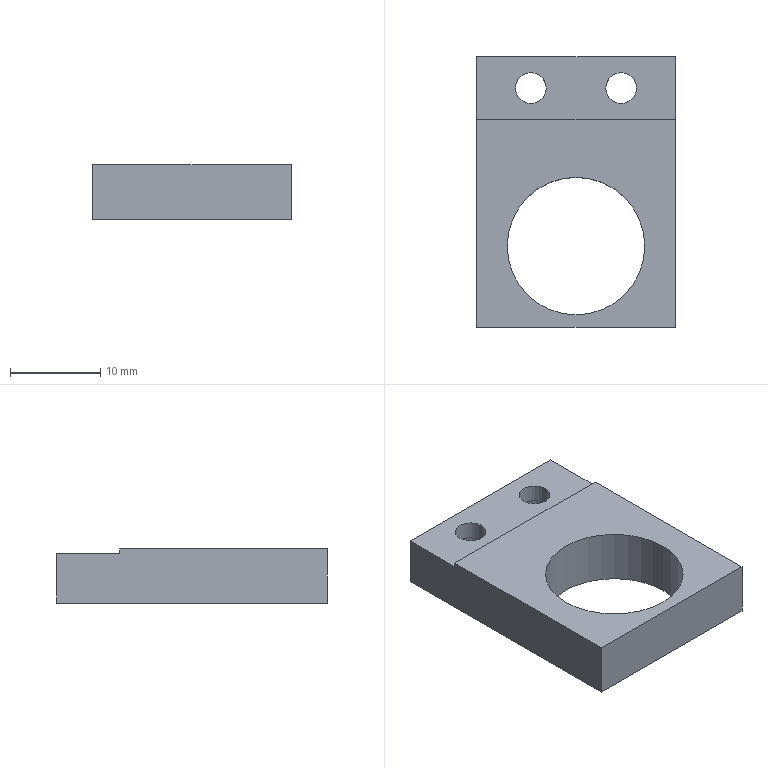Part | SolidWorks | features ICE 2, Extrusion 1 | 1 solid | 20 faces | box 22 x 30 x 6 mm | volume 2556 mm3 | cylinder 10 | plane 10 | commonest cylinder face diameters 3.4 x4 6 x4 15.23 x2
STEP:
#1=CARTESIAN_POINT('',(-0.003936,0.01062,0.0035));
#2=VERTEX_POINT('',#1);
#3=CARTESIAN_POINT('',(-0.009936,0.01062,0.0035));
#4=VERTEX_POINT('',#3);
#5=CARTESIAN_POINT('',(-0.006936,0.01062,0.0035));
#6=DIRECTION('',(0.,0.,-1.));
#7=DIRECTION('',(-1.,0.,0.));
#8=AXIS2_PLACEMENT_3D('',#5,#6,#7);
#9=CIRCLE('',#8,0.003);
#10=EDGE_CURVE('',#2,#4,#9,.T.);
#11=ORIENTED_EDGE('',*,*,#10,.F.);
#12=CARTESIAN_POINT('',(-0.003936,0.01062,0.));
#13=VERTEX_POINT('',#12);
#14=CARTESIAN_POINT('',(-0.003936,0.01062,0.0035));
#15=DIRECTION('',(0.,0.,-1.));
#16=VECTOR('',#15,1.);
#17=LINE('',#14,#16);
#18=EDGE_CURVE('',#2,#13,#17,.T.);
#19=ORIENTED_EDGE('',*,*,#18,.T.);
#20=CARTESIAN_POINT('',(-0.009936,0.01062,0.));
#21=VERTEX_POINT('',#20);
#22=CARTESIAN_POINT('',(-0.006936,0.01062,0.));
#23=DIRECTION('',(0.,0.,-1.));
#24=DIRECTION('',(-1.,0.,0.));
#25=AXIS2_PLACEMENT_3D('',#22,#23,#24);
#26=CIRCLE('',#25,0.003);
#27=EDGE_CURVE('',#13,#21,#26,.T.);
#28=ORIENTED_EDGE('',*,*,#27,.T.);
#29=CARTESIAN_POINT('',(-0.009936,0.01062,0.0035));
#30=DIRECTION('',(0.,0.,-1.));
#31=VECTOR('',#30,1.);
#32=LINE('',#29,#31);
#33=EDGE_CURVE('',#4,#21,#32,.T.);
#34=ORIENTED_EDGE('',*,*,#33,.F.);
#35=EDGE_LOOP('',(#11,#19,#28,#34));
#36=FACE_OUTER_BOUND('',#35,.T.);
#37=CARTESIAN_POINT('',(-0.006936,0.01062,0.0035));
#38=DIRECTION('',(0.,0.,-1.));
#39=DIRECTION('',(-1.,0.,0.));
#40=AXIS2_PLACEMENT_3D('',#37,#38,#39);
#41=CYLINDRICAL_SURFACE('',#40,0.003);
#42=ADVANCED_FACE('',(#36),#41,.F.);
#43=CARTESIAN_POINT('',(0.006064,0.01062,0.0035));
#44=VERTEX_POINT('',#43);
#45=CARTESIAN_POINT('',(0.00006422,0.01062,0.0035));
#46=VERTEX_POINT('',#45);
#47=CARTESIAN_POINT('',(0.003064,0.01062,0.0035));
#48=DIRECTION('',(0.,0.,-1.));
#49=DIRECTION('',(-1.,0.,0.));
#50=AXIS2_PLACEMENT_3D('',#47,#48,#49);
#51=CIRCLE('',#50,0.003);
#52=EDGE_CURVE('',#44,#46,#51,.T.);
#53=ORIENTED_EDGE('',*,*,#52,.F.);
#54=CARTESIAN_POINT('',(0.006064,0.01062,0.));
#55=VERTEX_POINT('',#54);
#56=CARTESIAN_POINT('',(0.006064,0.01062,0.0035));
#57=DIRECTION('',(0.,0.,-1.));
#58=VECTOR('',#57,1.);
#59=LINE('',#56,#58);
#60=EDGE_CURVE('',#44,#55,#59,.T.);
#61=ORIENTED_EDGE('',*,*,#60,.T.);
#62=CARTESIAN_POINT('',(0.00006422,0.01062,0.));
#63=VERTEX_POINT('',#62);
#64=CARTESIAN_POINT('',(0.003064,0.01062,0.));
#65=DIRECTION('',(0.,0.,-1.));
#66=DIRECTION('',(-1.,0.,0.));
#67=AXIS2_PLACEMENT_3D('',#64,#65,#66);
#68=CIRCLE('',#67,0.003);
#69=EDGE_CURVE('',#55,#63,#68,.T.);
#70=ORIENTED_EDGE('',*,*,#69,.T.);
#71=CARTESIAN_POINT('',(0.00006422,0.01062,0.0035));
#72=DIRECTION('',(0.,0.,-1.));
#73=VECTOR('',#72,1.);
#74=LINE('',#71,#73);
#75=EDGE_CURVE('',#46,#63,#74,.T.);
#76=ORIENTED_EDGE('',*,*,#75,.F.);
#77=EDGE_LOOP('',(#53,#61,#70,#76));
#78=FACE_OUTER_BOUND('',#77,.T.);
#79=CARTESIAN_POINT('',(0.003064,0.01062,0.0035));
#80=DIRECTION('',(0.,0.,-1.));
#81=DIRECTION('',(-1.,0.,0.));
#82=AXIS2_PLACEMENT_3D('',#79,#80,#81);
#83=CYLINDRICAL_SURFACE('',#82,0.003);
#84=ADVANCED_FACE('',(#78),#83,.F.);
#85=CARTESIAN_POINT('',(-0.009551,-0.006881,0.006));
#86=VERTEX_POINT('',#85);
#87=CARTESIAN_POINT('',(0.005679,-0.006881,0.006));
#88=VERTEX_POINT('',#87);
#89=CARTESIAN_POINT('',(-0.001936,-0.006881,0.006));
#90=DIRECTION('',(0.,0.,1.));
#91=DIRECTION('',(1.,0.,0.));
#92=AXIS2_PLACEMENT_3D('',#89,#90,#91);
#93=CIRCLE('',#92,0.007615);
#94=EDGE_CURVE('',#86,#88,#93,.T.);
#95=ORIENTED_EDGE('',*,*,#94,.T.);
#96=CARTESIAN_POINT('',(0.005679,-0.006881,0.));
#97=VERTEX_POINT('',#96);
#98=CARTESIAN_POINT('',(0.005679,-0.006881,0.006));
#99=DIRECTION('',(0.,0.,-1.));
#100=VECTOR('',#99,1.);
#101=LINE('',#98,#100);
#102=EDGE_CURVE('',#88,#97,#101,.T.);
#103=ORIENTED_EDGE('',*,*,#102,.T.);
#104=CARTESIAN_POINT('',(-0.009551,-0.006881,0.));
#105=VERTEX_POINT('',#104);
#106=CARTESIAN_POINT('',(-0.001936,-0.006881,0.));
#107=DIRECTION('',(0.,0.,1.));
#108=DIRECTION('',(1.,0.,0.));
#109=AXIS2_PLACEMENT_3D('',#106,#107,#108);
#110=CIRCLE('',#109,0.007615);
#111=EDGE_CURVE('',#105,#97,#110,.T.);
#112=ORIENTED_EDGE('',*,*,#111,.F.);
#113=CARTESIAN_POINT('',(-0.009551,-0.006881,0.006));
#114=DIRECTION('',(0.,0.,-1.));
#115=VECTOR('',#114,1.);
#116=LINE('',#113,#115);
#117=EDGE_CURVE('',#86,#105,#116,.T.);
#118=ORIENTED_EDGE('',*,*,#117,.F.);
#119=EDGE_LOOP('',(#95,#103,#112,#118));
#120=FACE_OUTER_BOUND('',#119,.T.);
#121=CARTESIAN_POINT('',(-0.001936,-0.006881,0.006));
#122=DIRECTION('',(0.,0.,-1.));
#123=DIRECTION('',(-1.,0.,0.));
#124=AXIS2_PLACEMENT_3D('',#121,#122,#123);
#125=CYLINDRICAL_SURFACE('',#124,0.007615);
#126=ADVANCED_FACE('',(#120),#125,.F.);
#127=CARTESIAN_POINT('',(0.004764,0.01062,0.0055));
#128=VERTEX_POINT('',#127);
#129=CARTESIAN_POINT('',(0.001364,0.01062,0.0055));
#130=VERTEX_POINT('',#129);
#131=CARTESIAN_POINT('',(0.003064,0.01062,0.0055));
#132=DIRECTION('',(0.,0.,-1.));
#133=DIRECTION('',(-1.,0.,0.));
#134=AXIS2_PLACEMENT_3D('',#131,#132,#133);
#135=CIRCLE('',#134,0.0017);
#136=EDGE_CURVE('',#128,#130,#135,.T.);
#137=ORIENTED_EDGE('',*,*,#136,.F.);
#138=CARTESIAN_POINT('',(0.004764,0.01062,0.0035));
#139=VERTEX_POINT('',#138);
#140=CARTESIAN_POINT('',(0.004764,0.01062,0.006));
#141=DIRECTION('',(0.,0.,-1.));
#142=VECTOR('',#141,1.);
#143=LINE('',#140,#142);
#144=EDGE_CURVE('',#128,#139,#143,.T.);
#145=ORIENTED_EDGE('',*,*,#144,.T.);
#146=CARTESIAN_POINT('',(0.001364,0.01062,0.0035));
#147=VERTEX_POINT('',#146);
#148=CARTESIAN_POINT('',(0.003064,0.01062,0.0035));
#149=DIRECTION('',(0.,0.,-1.));
#150=DIRECTION('',(-1.,0.,0.));
#151=AXIS2_PLACEMENT_3D('',#148,#149,#150);
#152=CIRCLE('',#151,0.0017);
#153=EDGE_CURVE('',#139,#147,#152,.T.);
#154=ORIENTED_EDGE('',*,*,#153,.T.);
#155=CARTESIAN_POINT('',(0.001364,0.01062,0.006));
#156=DIRECTION('',(0.,0.,-1.));
#157=VECTOR('',#156,1.);
#158=LINE('',#155,#157);
#159=EDGE_CURVE('',#130,#147,#158,.T.);
#160=ORIENTED_EDGE('',*,*,#159,.F.);
#161=EDGE_LOOP('',(#137,#145,#154,#160));
#162=FACE_OUTER_BOUND('',#161,.T.);
#163=CARTESIAN_POINT('',(0.003064,0.01062,0.006));
#164=DIRECTION('',(0.,0.,-1.));
#165=DIRECTION('',(-1.,0.,0.));
#166=AXIS2_PLACEMENT_3D('',#163,#164,#165);
#167=CYLINDRICAL_SURFACE('',#166,0.0017);
#168=ADVANCED_FACE('',(#162),#167,.F.);
#169=CARTESIAN_POINT('',(-0.005236,0.01062,0.0055));
#170=VERTEX_POINT('',#169);
#171=CARTESIAN_POINT('',(-0.008636,0.01062,0.0055));
#172=VERTEX_POINT('',#171);
#173=CARTESIAN_POINT('',(-0.006936,0.01062,0.0055));
#174=DIRECTION('',(0.,0.,-1.));
#175=DIRECTION('',(-1.,0.,0.));
#176=AXIS2_PLACEMENT_3D('',#173,#174,#175);
#177=CIRCLE('',#176,0.0017);
#178=EDGE_CURVE('',#170,#172,#177,.T.);
#179=ORIENTED_EDGE('',*,*,#178,.F.);
#180=CARTESIAN_POINT('',(-0.005236,0.01062,0.0035));
#181=VERTEX_POINT('',#180);
#182=CARTESIAN_POINT('',(-0.005236,0.01062,0.006));
#183=DIRECTION('',(0.,0.,-1.));
#184=VECTOR('',#183,1.);
#185=LINE('',#182,#184);
#186=EDGE_CURVE('',#170,#181,#185,.T.);
#187=ORIENTED_EDGE('',*,*,#186,.T.);
#188=CARTESIAN_POINT('',(-0.008636,0.01062,0.0035));
#189=VERTEX_POINT('',#188);
#190=CARTESIAN_POINT('',(-0.006936,0.01062,0.0035));
#191=DIRECTION('',(0.,0.,-1.));
#192=DIRECTION('',(-1.,0.,0.));
#193=AXIS2_PLACEMENT_3D('',#190,#191,#192);
#194=CIRCLE('',#193,0.0017);
#195=EDGE_CURVE('',#181,#189,#194,.T.);
#196=ORIENTED_EDGE('',*,*,#195,.T.);
#197=CARTESIAN_POINT('',(-0.008636,0.01062,0.006));
#198=DIRECTION('',(0.,0.,-1.));
#199=VECTOR('',#198,1.);
#200=LINE('',#197,#199);
#201=EDGE_CURVE('',#172,#189,#200,.T.);
#202=ORIENTED_EDGE('',*,*,#201,.F.);
#203=EDGE_LOOP('',(#179,#187,#196,#202));
#204=FACE_OUTER_BOUND('',#203,.T.);
#205=CARTESIAN_POINT('',(-0.006936,0.01062,0.006));
#206=DIRECTION('',(0.,0.,-1.));
#207=DIRECTION('',(-1.,0.,0.));
#208=AXIS2_PLACEMENT_3D('',#205,#206,#207);
#209=CYLINDRICAL_SURFACE('',#208,0.0017);
#210=ADVANCED_FACE('',(#204),#209,.F.);
#211=ORIENTED_EDGE('',*,*,#186,.F.);
#212=CARTESIAN_POINT('',(-0.006936,0.01062,0.0055));
#213=DIRECTION('',(0.,0.,-1.));
#214=DIRECTION('',(-1.,0.,0.));
#215=AXIS2_PLACEMENT_3D('',#212,#213,#214);
#216=CIRCLE('',#215,0.0017);
#217=EDGE_CURVE('',#172,#170,#216,.T.);
#218=ORIENTED_EDGE('',*,*,#217,.F.);
#219=ORIENTED_EDGE('',*,*,#201,.T.);
#220=CARTESIAN_POINT('',(-0.006936,0.01062,0.0035));
#221=DIRECTION('',(0.,0.,-1.));
#222=DIRECTION('',(-1.,0.,0.));
#223=AXIS2_PLACEMENT_3D('',#220,#221,#222);
#224=CIRCLE('',#223,0.0017);
#225=EDGE_CURVE('',#189,#181,#224,.T.);
#226=ORIENTED_EDGE('',*,*,#225,.T.);
#227=EDGE_LOOP('',(#211,#218,#219,#226));
#228=FACE_OUTER_BOUND('',#227,.T.);
#229=CARTESIAN_POINT('',(-0.006936,0.01062,0.006));
#230=DIRECTION('',(0.,0.,-1.));
#231=DIRECTION('',(-1.,0.,0.));
#232=AXIS2_PLACEMENT_3D('',#229,#230,#231);
#233=CYLINDRICAL_SURFACE('',#232,0.0017);
#234=ADVANCED_FACE('',(#228),#233,.F.);
#235=ORIENTED_EDGE('',*,*,#144,.F.);
#236=CARTESIAN_POINT('',(0.003064,0.01062,0.0055));
#237=DIRECTION('',(0.,0.,-1.));
#238=DIRECTION('',(-1.,0.,0.));
#239=AXIS2_PLACEMENT_3D('',#236,#237,#238);
#240=CIRCLE('',#239,0.0017);
#241=EDGE_CURVE('',#130,#128,#240,.T.);
#242=ORIENTED_EDGE('',*,*,#241,.F.);
#243=ORIENTED_EDGE('',*,*,#159,.T.);
#244=CARTESIAN_POINT('',(0.003064,0.01062,0.0035));
#245=DIRECTION('',(0.,0.,-1.));
#246=DIRECTION('',(-1.,0.,0.));
#247=AXIS2_PLACEMENT_3D('',#244,#245,#246);
#248=CIRCLE('',#247,0.0017);
#249=EDGE_CURVE('',#147,#139,#248,.T.);
#250=ORIENTED_EDGE('',*,*,#249,.T.);
#251=EDGE_LOOP('',(#235,#242,#243,#250));
#252=FACE_OUTER_BOUND('',#251,.T.);
#253=CARTESIAN_POINT('',(0.003064,0.01062,0.006));
#254=DIRECTION('',(0.,0.,-1.));
#255=DIRECTION('',(-1.,0.,0.));
#256=AXIS2_PLACEMENT_3D('',#253,#254,#255);
#257=CYLINDRICAL_SURFACE('',#256,0.0017);
#258=ADVANCED_FACE('',(#252),#257,.F.);
#259=CARTESIAN_POINT('',(0.009064,0.007119,0.006));
#260=VERTEX_POINT('',#259);
#261=CARTESIAN_POINT('',(-0.01294,0.007119,0.006));
#262=VERTEX_POINT('',#261);
#263=CARTESIAN_POINT('',(0.009064,0.007119,0.006));
#264=DIRECTION('',(-1.,0.,0.));
#265=VECTOR('',#264,1.);
#266=LINE('',#263,#265);
#267=EDGE_CURVE('',#260,#262,#266,.T.);
#268=ORIENTED_EDGE('',*,*,#267,.T.);
#269=CARTESIAN_POINT('',(-0.01294,-0.01588,0.006));
#270=VERTEX_POINT('',#269);
#271=CARTESIAN_POINT('',(-0.01294,0.01412,0.006));
#272=DIRECTION('',(0.,-1.,0.));
#273=VECTOR('',#272,1.);
#274=LINE('',#271,#273);
#275=EDGE_CURVE('',#262,#270,#274,.T.);
#276=ORIENTED_EDGE('',*,*,#275,.T.);
#277=CARTESIAN_POINT('',(0.009064,-0.01588,0.006));
#278=VERTEX_POINT('',#277);
#279=CARTESIAN_POINT('',(-0.01294,-0.01588,0.006));
#280=DIRECTION('',(1.,0.,0.));
#281=VECTOR('',#280,1.);
#282=LINE('',#279,#281);
#283=EDGE_CURVE('',#270,#278,#282,.T.);
#284=ORIENTED_EDGE('',*,*,#283,.T.);
#285=CARTESIAN_POINT('',(0.009064,0.01412,0.006));
#286=DIRECTION('',(0.,1.,0.));
#287=VECTOR('',#286,1.);
#288=LINE('',#285,#287);
#289=EDGE_CURVE('',#278,#260,#288,.T.);
#290=ORIENTED_EDGE('',*,*,#289,.T.);
#291=EDGE_LOOP('',(#268,#276,#284,#290));
#292=FACE_OUTER_BOUND('',#291,.T.);
#293=ORIENTED_EDGE('',*,*,#94,.F.);
#294=CARTESIAN_POINT('',(-0.001936,-0.006881,0.006));
#295=DIRECTION('',(0.,0.,1.));
#296=DIRECTION('',(1.,0.,0.));
#297=AXIS2_PLACEMENT_3D('',#294,#295,#296);
#298=CIRCLE('',#297,0.007615);
#299=EDGE_CURVE('',#88,#86,#298,.T.);
#300=ORIENTED_EDGE('',*,*,#299,.F.);
#301=EDGE_LOOP('',(#293,#300));
#302=FACE_BOUND('',#301,.T.);
#303=CARTESIAN_POINT('',(0.,0.,0.006));
#304=DIRECTION('',(0.,0.,1.));
#305=DIRECTION('',(1.,0.,0.));
#306=AXIS2_PLACEMENT_3D('',#303,#304,#305);
#307=PLANE('',#306);
#308=ADVANCED_FACE('',(#292,#302),#307,.T.);
#309=CARTESIAN_POINT('',(0.003064,0.01062,0.));
#310=DIRECTION('',(0.,0.,-1.));
#311=DIRECTION('',(-1.,0.,0.));
#312=AXIS2_PLACEMENT_3D('',#309,#310,#311);
#313=CIRCLE('',#312,0.003);
#314=EDGE_CURVE('',#63,#55,#313,.T.);
#315=ORIENTED_EDGE('',*,*,#314,.F.);
#316=ORIENTED_EDGE('',*,*,#69,.F.);
#317=EDGE_LOOP('',(#315,#316));
#318=FACE_BOUND('',#317,.T.);
#319=CARTESIAN_POINT('',(-0.006936,0.01062,0.));
#320=DIRECTION('',(0.,0.,-1.));
#321=DIRECTION('',(-1.,0.,0.));
#322=AXIS2_PLACEMENT_3D('',#319,#320,#321);
#323=CIRCLE('',#322,0.003);
#324=EDGE_CURVE('',#21,#13,#323,.T.);
#325=ORIENTED_EDGE('',*,*,#324,.F.);
#326=ORIENTED_EDGE('',*,*,#27,.F.);
#327=EDGE_LOOP('',(#325,#326));
#328=FACE_BOUND('',#327,.T.);
#329=CARTESIAN_POINT('',(-0.01294,0.01412,0.));
#330=VERTEX_POINT('',#329);
#331=CARTESIAN_POINT('',(-0.01294,-0.01588,0.));
#332=VERTEX_POINT('',#331);
#333=CARTESIAN_POINT('',(-0.01294,0.01412,0.));
#334=DIRECTION('',(0.,-1.,0.));
#335=VECTOR('',#334,1.);
#336=LINE('',#333,#335);
#337=EDGE_CURVE('',#330,#332,#336,.T.);
#338=ORIENTED_EDGE('',*,*,#337,.F.);
#339=CARTESIAN_POINT('',(0.009064,0.01412,0.));
#340=VERTEX_POINT('',#339);
#341=CARTESIAN_POINT('',(-0.01294,0.01412,0.));
#342=DIRECTION('',(-1.,0.,0.));
#343=VECTOR('',#342,1.);
#344=LINE('',#341,#343);
#345=EDGE_CURVE('',#340,#330,#344,.T.);
#346=ORIENTED_EDGE('',*,*,#345,.F.);
#347=CARTESIAN_POINT('',(0.009064,-0.01588,0.));
#348=VERTEX_POINT('',#347);
#349=CARTESIAN_POINT('',(0.009064,0.01412,0.));
#350=DIRECTION('',(0.,1.,0.));
#351=VECTOR('',#350,1.);
#352=LINE('',#349,#351);
#353=EDGE_CURVE('',#348,#340,#352,.T.);
#354=ORIENTED_EDGE('',*,*,#353,.F.);
#355=CARTESIAN_POINT('',(-0.01294,-0.01588,0.));
#356=DIRECTION('',(1.,0.,0.));
#357=VECTOR('',#356,1.);
#358=LINE('',#355,#357);
#359=EDGE_CURVE('',#332,#348,#358,.T.);
#360=ORIENTED_EDGE('',*,*,#359,.F.);
#361=EDGE_LOOP('',(#338,#346,#354,#360));
#362=FACE_OUTER_BOUND('',#361,.T.);
#363=ORIENTED_EDGE('',*,*,#111,.T.);
#364=CARTESIAN_POINT('',(-0.001936,-0.006881,0.));
#365=DIRECTION('',(0.,0.,1.));
#366=DIRECTION('',(1.,0.,0.));
#367=AXIS2_PLACEMENT_3D('',#364,#365,#366);
#368=CIRCLE('',#367,0.007615);
#369=EDGE_CURVE('',#97,#105,#368,.T.);
#370=ORIENTED_EDGE('',*,*,#369,.T.);
#371=EDGE_LOOP('',(#363,#370));
#372=FACE_BOUND('',#371,.T.);
#373=CARTESIAN_POINT('',(0.,0.,0.));
#374=DIRECTION('',(0.,0.,1.));
#375=DIRECTION('',(1.,0.,0.));
#376=AXIS2_PLACEMENT_3D('',#373,#374,#375);
#377=PLANE('',#376);
#378=ADVANCED_FACE('',(#318,#328,#362,#372),#377,.F.);
#379=ORIENTED_EDGE('',*,*,#275,.F.);
#380=CARTESIAN_POINT('',(-0.01294,0.007119,0.0055));
#381=VERTEX_POINT('',#380);
#382=CARTESIAN_POINT('',(-0.01294,0.007119,0.006));
#383=DIRECTION('',(0.,0.,1.));
#384=VECTOR('',#383,1.);
#385=LINE('',#382,#384);
#386=EDGE_CURVE('',#381,#262,#385,.T.);
#387=ORIENTED_EDGE('',*,*,#386,.F.);
#388=CARTESIAN_POINT('',(-0.01294,0.01412,0.0055));
#389=VERTEX_POINT('',#388);
#390=CARTESIAN_POINT('',(-0.01294,0.01412,0.0055));
#391=DIRECTION('',(0.,-1.,0.));
#392=VECTOR('',#391,1.);
#393=LINE('',#390,#392);
#394=EDGE_CURVE('',#389,#381,#393,.T.);
#395=ORIENTED_EDGE('',*,*,#394,.F.);
#396=CARTESIAN_POINT('',(-0.01294,0.01412,0.006));
#397=DIRECTION('',(0.,0.,-1.));
#398=VECTOR('',#397,1.);
#399=LINE('',#396,#398);
#400=EDGE_CURVE('',#389,#330,#399,.T.);
#401=ORIENTED_EDGE('',*,*,#400,.T.);
#402=ORIENTED_EDGE('',*,*,#337,.T.);
#403=CARTESIAN_POINT('',(-0.01294,-0.01588,0.006));
#404=DIRECTION('',(0.,0.,-1.));
#405=VECTOR('',#404,1.);
#406=LINE('',#403,#405);
#407=EDGE_CURVE('',#270,#332,#406,.T.);
#408=ORIENTED_EDGE('',*,*,#407,.F.);
#409=EDGE_LOOP('',(#379,#387,#395,#401,#402,#408));
#410=FACE_OUTER_BOUND('',#409,.T.);
#411=CARTESIAN_POINT('',(-0.01294,0.01412,0.006));
#412=DIRECTION('',(1.,0.,0.));
#413=DIRECTION('',(0.,0.,-1.));
#414=AXIS2_PLACEMENT_3D('',#411,#412,#413);
#415=PLANE('',#414);
#416=ADVANCED_FACE('',(#410),#415,.F.);
#417=ORIENTED_EDGE('',*,*,#359,.T.);
#418=CARTESIAN_POINT('',(0.009064,-0.01588,0.006));
#419=DIRECTION('',(0.,0.,-1.));
#420=VECTOR('',#419,1.);
#421=LINE('',#418,#420);
#422=EDGE_CURVE('',#278,#348,#421,.T.);
#423=ORIENTED_EDGE('',*,*,#422,.F.);
#424=ORIENTED_EDGE('',*,*,#283,.F.);
#425=ORIENTED_EDGE('',*,*,#407,.T.);
#426=EDGE_LOOP('',(#417,#423,#424,#425));
#427=FACE_OUTER_BOUND('',#426,.T.);
#428=CARTESIAN_POINT('',(-0.01294,-0.01588,0.006));
#429=DIRECTION('',(0.,1.,0.));
#430=DIRECTION('',(0.,0.,1.));
#431=AXIS2_PLACEMENT_3D('',#428,#429,#430);
#432=PLANE('',#431);
#433=ADVANCED_FACE('',(#427),#432,.F.);
#434=CARTESIAN_POINT('',(0.009064,0.01412,0.0055));
#435=VERTEX_POINT('',#434);
#436=CARTESIAN_POINT('',(0.009064,0.007119,0.0055));
#437=VERTEX_POINT('',#436);
#438=CARTESIAN_POINT('',(0.009064,0.01412,0.0055));
#439=DIRECTION('',(0.,-1.,0.));
#440=VECTOR('',#439,1.);
#441=LINE('',#438,#440);
#442=EDGE_CURVE('',#435,#437,#441,.T.);
#443=ORIENTED_EDGE('',*,*,#442,.T.);
#444=CARTESIAN_POINT('',(0.009064,0.007119,0.006));
#445=DIRECTION('',(0.,0.,1.));
#446=VECTOR('',#445,1.);
#447=LINE('',#444,#446);
#448=EDGE_CURVE('',#437,#260,#447,.T.);
#449=ORIENTED_EDGE('',*,*,#448,.T.);
#450=ORIENTED_EDGE('',*,*,#289,.F.);
#451=ORIENTED_EDGE('',*,*,#422,.T.);
#452=ORIENTED_EDGE('',*,*,#353,.T.);
#453=CARTESIAN_POINT('',(0.009064,0.01412,0.006));
#454=DIRECTION('',(0.,0.,-1.));
#455=VECTOR('',#454,1.);
#456=LINE('',#453,#455);
#457=EDGE_CURVE('',#435,#340,#456,.T.);
#458=ORIENTED_EDGE('',*,*,#457,.F.);
#459=EDGE_LOOP('',(#443,#449,#450,#451,#452,#458));
#460=FACE_OUTER_BOUND('',#459,.T.);
#461=CARTESIAN_POINT('',(0.009064,0.01412,0.006));
#462=DIRECTION('',(-1.,0.,0.));
#463=DIRECTION('',(0.,-1.,0.));
#464=AXIS2_PLACEMENT_3D('',#461,#462,#463);
#465=PLANE('',#464);
#466=ADVANCED_FACE('',(#460),#465,.F.);
#467=ORIENTED_EDGE('',*,*,#400,.F.);
#468=CARTESIAN_POINT('',(0.009064,0.01412,0.0055));
#469=DIRECTION('',(-1.,0.,0.));
#470=VECTOR('',#469,1.);
#471=LINE('',#468,#470);
#472=EDGE_CURVE('',#435,#389,#471,.T.);
#473=ORIENTED_EDGE('',*,*,#472,.F.);
#474=ORIENTED_EDGE('',*,*,#457,.T.);
#475=ORIENTED_EDGE('',*,*,#345,.T.);
#476=EDGE_LOOP('',(#467,#473,#474,#475));
#477=FACE_OUTER_BOUND('',#476,.T.);
#478=CARTESIAN_POINT('',(-0.01294,0.01412,0.006));
#479=DIRECTION('',(0.,-1.,0.));
#480=DIRECTION('',(0.,0.,-1.));
#481=AXIS2_PLACEMENT_3D('',#478,#479,#480);
#482=PLANE('',#481);
#483=ADVANCED_FACE('',(#477),#482,.F.);
#484=ORIENTED_EDGE('',*,*,#102,.F.);
#485=ORIENTED_EDGE('',*,*,#299,.T.);
#486=ORIENTED_EDGE('',*,*,#117,.T.);
#487=ORIENTED_EDGE('',*,*,#369,.F.);
#488=EDGE_LOOP('',(#484,#485,#486,#487));
#489=FACE_OUTER_BOUND('',#488,.T.);
#490=CARTESIAN_POINT('',(-0.001936,-0.006881,0.006));
#491=DIRECTION('',(0.,0.,-1.));
#492=DIRECTION('',(-1.,0.,0.));
#493=AXIS2_PLACEMENT_3D('',#490,#491,#492);
#494=CYLINDRICAL_SURFACE('',#493,0.007615);
#495=ADVANCED_FACE('',(#489),#494,.F.);
#496=ORIENTED_EDGE('',*,*,#386,.T.);
#497=ORIENTED_EDGE('',*,*,#267,.F.);
#498=ORIENTED_EDGE('',*,*,#448,.F.);
#499=CARTESIAN_POINT('',(0.009064,0.007119,0.0055));
#500=DIRECTION('',(-1.,0.,0.));
#501=VECTOR('',#500,1.);
#502=LINE('',#499,#501);
#503=EDGE_CURVE('',#437,#381,#502,.T.);
#504=ORIENTED_EDGE('',*,*,#503,.T.);
#505=EDGE_LOOP('',(#496,#497,#498,#504));
#506=FACE_OUTER_BOUND('',#505,.T.);
#507=CARTESIAN_POINT('',(0.009064,0.007119,0.006));
#508=DIRECTION('',(0.,-1.,0.));
#509=DIRECTION('',(0.,0.,-1.));
#510=AXIS2_PLACEMENT_3D('',#507,#508,#509);
#511=PLANE('',#510);
#512=ADVANCED_FACE('',(#506),#511,.F.);
#513=ORIENTED_EDGE('',*,*,#217,.T.);
#514=ORIENTED_EDGE('',*,*,#178,.T.);
#515=EDGE_LOOP('',(#513,#514));
#516=FACE_BOUND('',#515,.T.);
#517=ORIENTED_EDGE('',*,*,#241,.T.);
#518=ORIENTED_EDGE('',*,*,#136,.T.);
#519=EDGE_LOOP('',(#517,#518));
#520=FACE_BOUND('',#519,.T.);
#521=ORIENTED_EDGE('',*,*,#394,.T.);
#522=ORIENTED_EDGE('',*,*,#503,.F.);
#523=ORIENTED_EDGE('',*,*,#442,.F.);
#524=ORIENTED_EDGE('',*,*,#472,.T.);
#525=EDGE_LOOP('',(#521,#522,#523,#524));
#526=FACE_OUTER_BOUND('',#525,.T.);
#527=CARTESIAN_POINT('',(0.009064,0.01412,0.0055));
#528=DIRECTION('',(0.,0.,-1.));
#529=DIRECTION('',(-1.,0.,0.));
#530=AXIS2_PLACEMENT_3D('',#527,#528,#529);
#531=PLANE('',#530);
#532=ADVANCED_FACE('',(#516,#520,#526),#531,.F.);
#533=ORIENTED_EDGE('',*,*,#60,.F.);
#534=CARTESIAN_POINT('',(0.003064,0.01062,0.0035));
#535=DIRECTION('',(0.,0.,-1.));
#536=DIRECTION('',(-1.,0.,0.));
#537=AXIS2_PLACEMENT_3D('',#534,#535,#536);
#538=CIRCLE('',#537,0.003);
#539=EDGE_CURVE('',#46,#44,#538,.T.);
#540=ORIENTED_EDGE('',*,*,#539,.F.);
#541=ORIENTED_EDGE('',*,*,#75,.T.);
#542=ORIENTED_EDGE('',*,*,#314,.T.);
#543=EDGE_LOOP('',(#533,#540,#541,#542));
#544=FACE_OUTER_BOUND('',#543,.T.);
#545=CARTESIAN_POINT('',(0.003064,0.01062,0.0035));
#546=DIRECTION('',(0.,0.,-1.));
#547=DIRECTION('',(-1.,0.,0.));
#548=AXIS2_PLACEMENT_3D('',#545,#546,#547);
#549=CYLINDRICAL_SURFACE('',#548,0.003);
#550=ADVANCED_FACE('',(#544),#549,.F.);
#551=ORIENTED_EDGE('',*,*,#249,.F.);
#552=ORIENTED_EDGE('',*,*,#153,.F.);
#553=EDGE_LOOP('',(#551,#552));
#554=FACE_BOUND('',#553,.T.);
#555=ORIENTED_EDGE('',*,*,#539,.T.);
#556=ORIENTED_EDGE('',*,*,#52,.T.);
#557=EDGE_LOOP('',(#555,#556));
#558=FACE_OUTER_BOUND('',#557,.T.);
#559=CARTESIAN_POINT('',(0.003064,0.01062,0.0035));
#560=DIRECTION('',(0.,0.,-1.));
#561=DIRECTION('',(-1.,0.,0.));
#562=AXIS2_PLACEMENT_3D('',#559,#560,#561);
#563=PLANE('',#562);
#564=ADVANCED_FACE('',(#554,#558),#563,.T.);
#565=ORIENTED_EDGE('',*,*,#18,.F.);
#566=CARTESIAN_POINT('',(-0.006936,0.01062,0.0035));
#567=DIRECTION('',(0.,0.,-1.));
#568=DIRECTION('',(-1.,0.,0.));
#569=AXIS2_PLACEMENT_3D('',#566,#567,#568);
#570=CIRCLE('',#569,0.003);
#571=EDGE_CURVE('',#4,#2,#570,.T.);
#572=ORIENTED_EDGE('',*,*,#571,.F.);
#573=ORIENTED_EDGE('',*,*,#33,.T.);
#574=ORIENTED_EDGE('',*,*,#324,.T.);
#575=EDGE_LOOP('',(#565,#572,#573,#574));
#576=FACE_OUTER_BOUND('',#575,.T.);
#577=CARTESIAN_POINT('',(-0.006936,0.01062,0.0035));
#578=DIRECTION('',(0.,0.,-1.));
#579=DIRECTION('',(-1.,0.,0.));
#580=AXIS2_PLACEMENT_3D('',#577,#578,#579);
#581=CYLINDRICAL_SURFACE('',#580,0.003);
#582=ADVANCED_FACE('',(#576),#581,.F.);
#583=ORIENTED_EDGE('',*,*,#225,.F.);
#584=ORIENTED_EDGE('',*,*,#195,.F.);
#585=EDGE_LOOP('',(#583,#584));
#586=FACE_BOUND('',#585,.T.);
#587=ORIENTED_EDGE('',*,*,#571,.T.);
#588=ORIENTED_EDGE('',*,*,#10,.T.);
#589=EDGE_LOOP('',(#587,#588));
#590=FACE_OUTER_BOUND('',#589,.T.);
#591=CARTESIAN_POINT('',(-0.006936,0.01062,0.0035));
#592=DIRECTION('',(0.,0.,-1.));
#593=DIRECTION('',(-1.,0.,0.));
#594=AXIS2_PLACEMENT_3D('',#591,#592,#593);
#595=PLANE('',#594);
#596=ADVANCED_FACE('',(#586,#590),#595,.T.);
#597=CLOSED_SHELL('',(#42,#84,#126,#168,#210,#234,#258,#308,#378,#416,#433,#466,#483,#495,#512,#532,#550,#564,#582,#596));
#598=MANIFOLD_SOLID_BREP('',#597);
#599=CARTESIAN_POINT('',(0.,0.,0.));
#600=DIRECTION('',(0.,0.,1.));
#601=DIRECTION('',(1.,0.,0.));
#602=AXIS2_PLACEMENT_3D('',#599,#600,#601);
#603=(LENGTH_UNIT()NAMED_UNIT(*)SI_UNIT($,.METRE.));
#604=UNCERTAINTY_MEASURE_WITH_UNIT(LENGTH_MEASURE(0.00001),#603,'','');
#605=(NAMED_UNIT(*)PLANE_ANGLE_UNIT()SI_UNIT($,.RADIAN.));
#606=(NAMED_UNIT(*)SI_UNIT($,.STERADIAN.)SOLID_ANGLE_UNIT());
#607=(GEOMETRIC_REPRESENTATION_CONTEXT(3)GLOBAL_UNCERTAINTY_ASSIGNED_CONTEXT((#604))GLOBAL_UNIT_ASSIGNED_CONTEXT((#603,#605,#606))REPRESENTATION_CONTEXT('',''));
#608=ADVANCED_BREP_SHAPE_REPRESENTATION('',(#598,#602),#607);